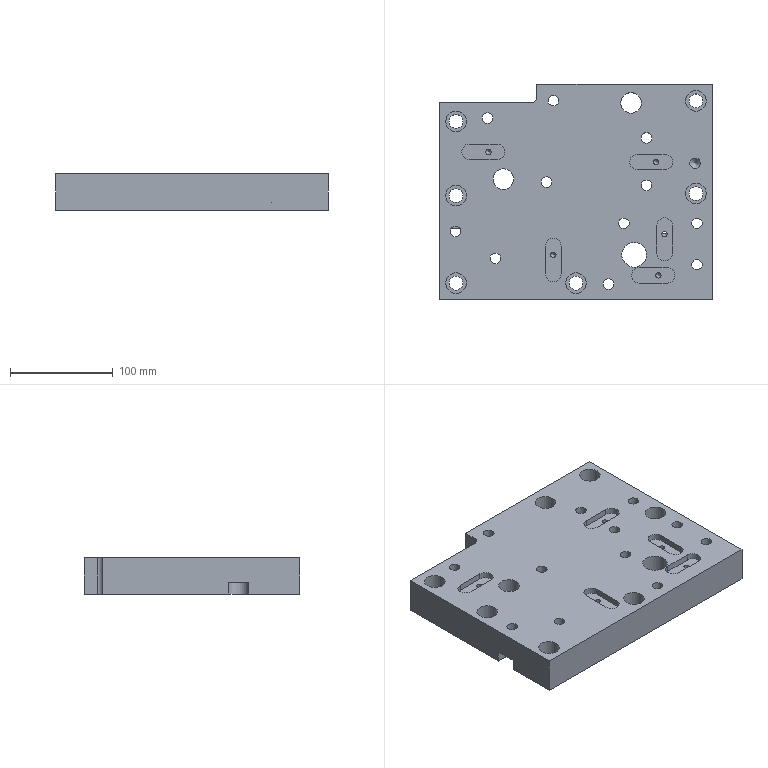Part | NX | features solid 2 | 1 solid | 91 faces | box 265 x 209 x 35 mm | volume 1701191 mm3 | cylinder 46 | plane 39 | cone 6 | commonest cylinder face diameters 10.3 x12 20 x11 15 x10 13.5 x6 5.2 x5 10 x1